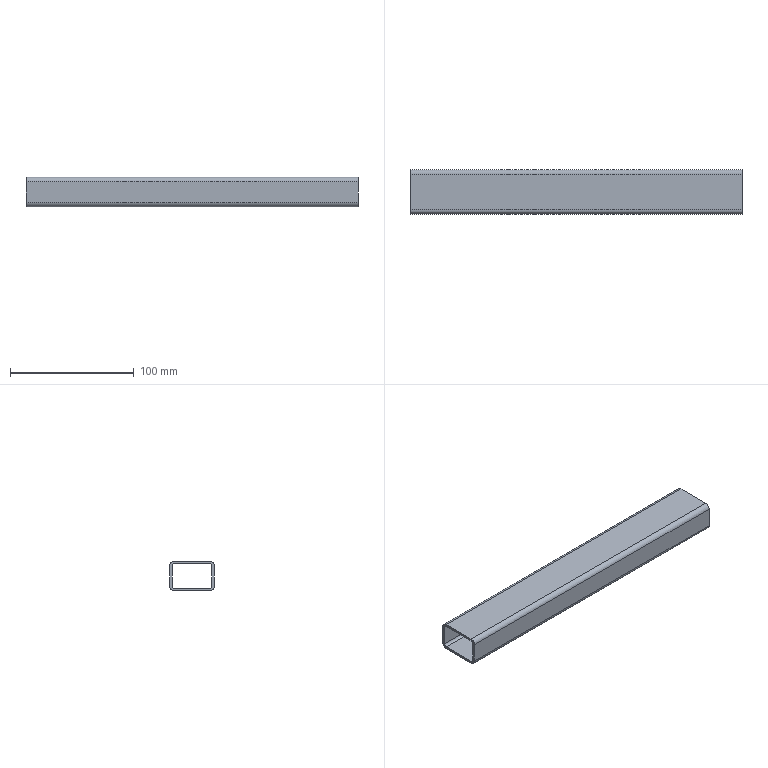Part | NX | 1 solid | 18 faces | box 268.32 x 36 x 24 mm | volume 55317 mm3 | plane 10 | cylinder 8 | commonest cylinder face diameters 3.84 x4 7.68 x4
STEP:
#1=CARTESIAN_POINT('',(264.834,-617.339,631.953));
#2=VERTEX_POINT('',#1);
#3=CARTESIAN_POINT('',(264.834,-613.499,628.113));
#4=VERTEX_POINT('',#3);
#5=CARTESIAN_POINT('',(264.834,-617.339,628.113));
#6=DIRECTION('',(-1.,0.,0.));
#7=DIRECTION('',(0.,0.,1.));
#8=AXIS2_PLACEMENT_3D('',#5,#6,#7);
#9=CIRCLE('',#8,3.84);
#10=EDGE_CURVE('',#2,#4,#9,.T.);
#11=ORIENTED_EDGE('',*,*,#10,.T.);
#12=CARTESIAN_POINT('',(-3.486,-613.499,628.113));
#13=VERTEX_POINT('',#12);
#14=CARTESIAN_POINT('',(-3.486,-613.499,628.113));
#15=DIRECTION('',(1.,0.,0.));
#16=VECTOR('',#15,1.);
#17=LINE('',#14,#16);
#18=EDGE_CURVE('',#13,#4,#17,.T.);
#19=ORIENTED_EDGE('',*,*,#18,.F.);
#20=CARTESIAN_POINT('',(-3.486,-617.339,631.953));
#21=VERTEX_POINT('',#20);
#22=CARTESIAN_POINT('',(-3.486,-617.339,628.113));
#23=DIRECTION('',(-1.,0.,0.));
#24=DIRECTION('',(0.,0.,1.));
#25=AXIS2_PLACEMENT_3D('',#22,#23,#24);
#26=CIRCLE('',#25,3.84);
#27=EDGE_CURVE('',#21,#13,#26,.T.);
#28=ORIENTED_EDGE('',*,*,#27,.F.);
#29=CARTESIAN_POINT('',(-3.486,-617.339,631.953));
#30=DIRECTION('',(1.,0.,0.));
#31=VECTOR('',#30,1.);
#32=LINE('',#29,#31);
#33=EDGE_CURVE('',#21,#2,#32,.T.);
#34=ORIENTED_EDGE('',*,*,#33,.T.);
#35=EDGE_LOOP('',(#11,#19,#28,#34));
#36=FACE_OUTER_BOUND('',#35,.T.);
#37=CARTESIAN_POINT('',(-3.486,-617.339,628.113));
#38=DIRECTION('',(1.,0.,0.));
#39=DIRECTION('',(0.,0.,-1.));
#40=AXIS2_PLACEMENT_3D('',#37,#38,#39);
#41=CYLINDRICAL_SURFACE('',#40,3.84);
#42=ADVANCED_FACE('',(#36),#41,.T.);
#43=CARTESIAN_POINT('',(264.834,-613.499,611.793));
#44=VERTEX_POINT('',#43);
#45=CARTESIAN_POINT('',(264.834,-613.499,628.113));
#46=DIRECTION('',(0.,0.,-1.));
#47=VECTOR('',#46,1.);
#48=LINE('',#45,#47);
#49=EDGE_CURVE('',#4,#44,#48,.T.);
#50=ORIENTED_EDGE('',*,*,#49,.T.);
#51=CARTESIAN_POINT('',(-3.486,-613.499,611.793));
#52=VERTEX_POINT('',#51);
#53=CARTESIAN_POINT('',(-3.486,-613.499,611.793));
#54=DIRECTION('',(1.,0.,0.));
#55=VECTOR('',#54,1.);
#56=LINE('',#53,#55);
#57=EDGE_CURVE('',#52,#44,#56,.T.);
#58=ORIENTED_EDGE('',*,*,#57,.F.);
#59=CARTESIAN_POINT('',(-3.486,-613.499,628.113));
#60=DIRECTION('',(0.,0.,-1.));
#61=VECTOR('',#60,1.);
#62=LINE('',#59,#61);
#63=EDGE_CURVE('',#13,#52,#62,.T.);
#64=ORIENTED_EDGE('',*,*,#63,.F.);
#65=ORIENTED_EDGE('',*,*,#18,.T.);
#66=EDGE_LOOP('',(#50,#58,#64,#65));
#67=FACE_OUTER_BOUND('',#66,.T.);
#68=CARTESIAN_POINT('',(-3.486,-613.499,628.113));
#69=DIRECTION('',(0.,-1.,0.));
#70=DIRECTION('',(0.,0.,-1.));
#71=AXIS2_PLACEMENT_3D('',#68,#69,#70);
#72=PLANE('',#71);
#73=ADVANCED_FACE('',(#67),#72,.F.);
#74=CARTESIAN_POINT('',(264.834,-617.339,607.953));
#75=VERTEX_POINT('',#74);
#76=CARTESIAN_POINT('',(264.834,-617.339,611.793));
#77=DIRECTION('',(-1.,0.,0.));
#78=DIRECTION('',(0.,0.,1.));
#79=AXIS2_PLACEMENT_3D('',#76,#77,#78);
#80=CIRCLE('',#79,3.84);
#81=EDGE_CURVE('',#44,#75,#80,.T.);
#82=ORIENTED_EDGE('',*,*,#81,.T.);
#83=CARTESIAN_POINT('',(-3.486,-617.339,607.953));
#84=VERTEX_POINT('',#83);
#85=CARTESIAN_POINT('',(-3.486,-617.339,607.953));
#86=DIRECTION('',(1.,0.,0.));
#87=VECTOR('',#86,1.);
#88=LINE('',#85,#87);
#89=EDGE_CURVE('',#84,#75,#88,.T.);
#90=ORIENTED_EDGE('',*,*,#89,.F.);
#91=CARTESIAN_POINT('',(-3.486,-617.339,611.793));
#92=DIRECTION('',(-1.,0.,0.));
#93=DIRECTION('',(0.,0.,1.));
#94=AXIS2_PLACEMENT_3D('',#91,#92,#93);
#95=CIRCLE('',#94,3.84);
#96=EDGE_CURVE('',#52,#84,#95,.T.);
#97=ORIENTED_EDGE('',*,*,#96,.F.);
#98=ORIENTED_EDGE('',*,*,#57,.T.);
#99=EDGE_LOOP('',(#82,#90,#97,#98));
#100=FACE_OUTER_BOUND('',#99,.T.);
#101=CARTESIAN_POINT('',(-3.486,-617.339,611.793));
#102=DIRECTION('',(1.,0.,0.));
#103=DIRECTION('',(0.,0.,-1.));
#104=AXIS2_PLACEMENT_3D('',#101,#102,#103);
#105=CYLINDRICAL_SURFACE('',#104,3.84);
#106=ADVANCED_FACE('',(#100),#105,.T.);
#107=CARTESIAN_POINT('',(264.834,-645.659,607.953));
#108=VERTEX_POINT('',#107);
#109=CARTESIAN_POINT('',(264.834,-645.659,607.953));
#110=DIRECTION('',(0.,-1.,0.));
#111=VECTOR('',#110,1.);
#112=LINE('',#109,#111);
#113=EDGE_CURVE('',#75,#108,#112,.T.);
#114=ORIENTED_EDGE('',*,*,#113,.T.);
#115=CARTESIAN_POINT('',(-3.486,-645.659,607.953));
#116=VERTEX_POINT('',#115);
#117=CARTESIAN_POINT('',(-3.486,-645.659,607.953));
#118=DIRECTION('',(1.,0.,0.));
#119=VECTOR('',#118,1.);
#120=LINE('',#117,#119);
#121=EDGE_CURVE('',#116,#108,#120,.T.);
#122=ORIENTED_EDGE('',*,*,#121,.F.);
#123=CARTESIAN_POINT('',(-3.486,-645.659,607.953));
#124=DIRECTION('',(0.,-1.,0.));
#125=VECTOR('',#124,1.);
#126=LINE('',#123,#125);
#127=EDGE_CURVE('',#84,#116,#126,.T.);
#128=ORIENTED_EDGE('',*,*,#127,.F.);
#129=ORIENTED_EDGE('',*,*,#89,.T.);
#130=EDGE_LOOP('',(#114,#122,#128,#129));
#131=FACE_OUTER_BOUND('',#130,.T.);
#132=CARTESIAN_POINT('',(-3.486,-645.659,607.953));
#133=DIRECTION('',(0.,0.,1.));
#134=DIRECTION('',(1.,0.,0.));
#135=AXIS2_PLACEMENT_3D('',#132,#133,#134);
#136=PLANE('',#135);
#137=ADVANCED_FACE('',(#131),#136,.F.);
#138=CARTESIAN_POINT('',(264.834,-649.499,611.793));
#139=VERTEX_POINT('',#138);
#140=CARTESIAN_POINT('',(264.834,-645.659,611.793));
#141=DIRECTION('',(-1.,0.,0.));
#142=DIRECTION('',(0.,0.,1.));
#143=AXIS2_PLACEMENT_3D('',#140,#141,#142);
#144=CIRCLE('',#143,3.84);
#145=EDGE_CURVE('',#108,#139,#144,.T.);
#146=ORIENTED_EDGE('',*,*,#145,.T.);
#147=CARTESIAN_POINT('',(-3.486,-649.499,611.793));
#148=VERTEX_POINT('',#147);
#149=CARTESIAN_POINT('',(-3.486,-649.499,611.793));
#150=DIRECTION('',(1.,0.,0.));
#151=VECTOR('',#150,1.);
#152=LINE('',#149,#151);
#153=EDGE_CURVE('',#148,#139,#152,.T.);
#154=ORIENTED_EDGE('',*,*,#153,.F.);
#155=CARTESIAN_POINT('',(-3.486,-645.659,611.793));
#156=DIRECTION('',(-1.,0.,0.));
#157=DIRECTION('',(0.,0.,1.));
#158=AXIS2_PLACEMENT_3D('',#155,#156,#157);
#159=CIRCLE('',#158,3.84);
#160=EDGE_CURVE('',#116,#148,#159,.T.);
#161=ORIENTED_EDGE('',*,*,#160,.F.);
#162=ORIENTED_EDGE('',*,*,#121,.T.);
#163=EDGE_LOOP('',(#146,#154,#161,#162));
#164=FACE_OUTER_BOUND('',#163,.T.);
#165=CARTESIAN_POINT('',(-3.486,-645.659,611.793));
#166=DIRECTION('',(1.,0.,0.));
#167=DIRECTION('',(0.,0.,-1.));
#168=AXIS2_PLACEMENT_3D('',#165,#166,#167);
#169=CYLINDRICAL_SURFACE('',#168,3.84);
#170=ADVANCED_FACE('',(#164),#169,.T.);
#171=CARTESIAN_POINT('',(264.834,-649.499,628.113));
#172=VERTEX_POINT('',#171);
#173=CARTESIAN_POINT('',(264.834,-649.499,611.793));
#174=DIRECTION('',(0.,0.,1.));
#175=VECTOR('',#174,1.);
#176=LINE('',#173,#175);
#177=EDGE_CURVE('',#139,#172,#176,.T.);
#178=ORIENTED_EDGE('',*,*,#177,.T.);
#179=CARTESIAN_POINT('',(-3.486,-649.499,628.113));
#180=VERTEX_POINT('',#179);
#181=CARTESIAN_POINT('',(-3.486,-649.499,628.113));
#182=DIRECTION('',(1.,0.,0.));
#183=VECTOR('',#182,1.);
#184=LINE('',#181,#183);
#185=EDGE_CURVE('',#180,#172,#184,.T.);
#186=ORIENTED_EDGE('',*,*,#185,.F.);
#187=CARTESIAN_POINT('',(-3.486,-649.499,611.793));
#188=DIRECTION('',(0.,0.,1.));
#189=VECTOR('',#188,1.);
#190=LINE('',#187,#189);
#191=EDGE_CURVE('',#148,#180,#190,.T.);
#192=ORIENTED_EDGE('',*,*,#191,.F.);
#193=ORIENTED_EDGE('',*,*,#153,.T.);
#194=EDGE_LOOP('',(#178,#186,#192,#193));
#195=FACE_OUTER_BOUND('',#194,.T.);
#196=CARTESIAN_POINT('',(-3.486,-649.499,611.793));
#197=DIRECTION('',(0.,1.,0.));
#198=DIRECTION('',(0.,0.,1.));
#199=AXIS2_PLACEMENT_3D('',#196,#197,#198);
#200=PLANE('',#199);
#201=ADVANCED_FACE('',(#195),#200,.F.);
#202=CARTESIAN_POINT('',(264.834,-645.659,631.953));
#203=VERTEX_POINT('',#202);
#204=CARTESIAN_POINT('',(264.834,-645.659,628.113));
#205=DIRECTION('',(-1.,0.,0.));
#206=DIRECTION('',(0.,0.,1.));
#207=AXIS2_PLACEMENT_3D('',#204,#205,#206);
#208=CIRCLE('',#207,3.84);
#209=EDGE_CURVE('',#172,#203,#208,.T.);
#210=ORIENTED_EDGE('',*,*,#209,.T.);
#211=CARTESIAN_POINT('',(-3.486,-645.659,631.953));
#212=VERTEX_POINT('',#211);
#213=CARTESIAN_POINT('',(-3.486,-645.659,631.953));
#214=DIRECTION('',(1.,0.,0.));
#215=VECTOR('',#214,1.);
#216=LINE('',#213,#215);
#217=EDGE_CURVE('',#212,#203,#216,.T.);
#218=ORIENTED_EDGE('',*,*,#217,.F.);
#219=CARTESIAN_POINT('',(-3.486,-645.659,628.113));
#220=DIRECTION('',(-1.,0.,0.));
#221=DIRECTION('',(0.,0.,1.));
#222=AXIS2_PLACEMENT_3D('',#219,#220,#221);
#223=CIRCLE('',#222,3.84);
#224=EDGE_CURVE('',#180,#212,#223,.T.);
#225=ORIENTED_EDGE('',*,*,#224,.F.);
#226=ORIENTED_EDGE('',*,*,#185,.T.);
#227=EDGE_LOOP('',(#210,#218,#225,#226));
#228=FACE_OUTER_BOUND('',#227,.T.);
#229=CARTESIAN_POINT('',(-3.486,-645.659,628.113));
#230=DIRECTION('',(1.,0.,0.));
#231=DIRECTION('',(0.,0.,-1.));
#232=AXIS2_PLACEMENT_3D('',#229,#230,#231);
#233=CYLINDRICAL_SURFACE('',#232,3.84);
#234=ADVANCED_FACE('',(#228),#233,.T.);
#235=CARTESIAN_POINT('',(264.834,-615.419,611.793));
#236=VERTEX_POINT('',#235);
#237=CARTESIAN_POINT('',(264.834,-617.339,609.873));
#238=VERTEX_POINT('',#237);
#239=CARTESIAN_POINT('',(264.834,-617.339,611.793));
#240=DIRECTION('',(-1.,0.,0.));
#241=DIRECTION('',(0.,0.,1.));
#242=AXIS2_PLACEMENT_3D('',#239,#240,#241);
#243=CIRCLE('',#242,1.92);
#244=EDGE_CURVE('',#236,#238,#243,.T.);
#245=ORIENTED_EDGE('',*,*,#244,.F.);
#246=CARTESIAN_POINT('',(-3.486,-615.419,611.793));
#247=VERTEX_POINT('',#246);
#248=CARTESIAN_POINT('',(-3.486,-615.419,611.793));
#249=DIRECTION('',(1.,0.,0.));
#250=VECTOR('',#249,1.);
#251=LINE('',#248,#250);
#252=EDGE_CURVE('',#247,#236,#251,.T.);
#253=ORIENTED_EDGE('',*,*,#252,.F.);
#254=CARTESIAN_POINT('',(-3.486,-617.339,609.873));
#255=VERTEX_POINT('',#254);
#256=CARTESIAN_POINT('',(-3.486,-617.339,611.793));
#257=DIRECTION('',(-1.,0.,0.));
#258=DIRECTION('',(0.,0.,1.));
#259=AXIS2_PLACEMENT_3D('',#256,#257,#258);
#260=CIRCLE('',#259,1.92);
#261=EDGE_CURVE('',#247,#255,#260,.T.);
#262=ORIENTED_EDGE('',*,*,#261,.T.);
#263=CARTESIAN_POINT('',(-3.486,-617.339,609.873));
#264=DIRECTION('',(1.,0.,0.));
#265=VECTOR('',#264,1.);
#266=LINE('',#263,#265);
#267=EDGE_CURVE('',#255,#238,#266,.T.);
#268=ORIENTED_EDGE('',*,*,#267,.T.);
#269=EDGE_LOOP('',(#245,#253,#262,#268));
#270=FACE_OUTER_BOUND('',#269,.T.);
#271=CARTESIAN_POINT('',(-3.486,-617.339,611.793));
#272=DIRECTION('',(1.,0.,0.));
#273=DIRECTION('',(0.,0.,-1.));
#274=AXIS2_PLACEMENT_3D('',#271,#272,#273);
#275=CYLINDRICAL_SURFACE('',#274,1.92);
#276=ADVANCED_FACE('',(#270),#275,.F.);
#277=CARTESIAN_POINT('',(264.834,-615.419,628.113));
#278=VERTEX_POINT('',#277);
#279=CARTESIAN_POINT('',(264.834,-615.419,628.113));
#280=DIRECTION('',(0.,0.,-1.));
#281=VECTOR('',#280,1.);
#282=LINE('',#279,#281);
#283=EDGE_CURVE('',#278,#236,#282,.T.);
#284=ORIENTED_EDGE('',*,*,#283,.F.);
#285=CARTESIAN_POINT('',(-3.486,-615.419,628.113));
#286=VERTEX_POINT('',#285);
#287=CARTESIAN_POINT('',(-3.486,-615.419,628.113));
#288=DIRECTION('',(1.,0.,0.));
#289=VECTOR('',#288,1.);
#290=LINE('',#287,#289);
#291=EDGE_CURVE('',#286,#278,#290,.T.);
#292=ORIENTED_EDGE('',*,*,#291,.F.);
#293=CARTESIAN_POINT('',(-3.486,-615.419,628.113));
#294=DIRECTION('',(0.,0.,-1.));
#295=VECTOR('',#294,1.);
#296=LINE('',#293,#295);
#297=EDGE_CURVE('',#286,#247,#296,.T.);
#298=ORIENTED_EDGE('',*,*,#297,.T.);
#299=ORIENTED_EDGE('',*,*,#252,.T.);
#300=EDGE_LOOP('',(#284,#292,#298,#299));
#301=FACE_OUTER_BOUND('',#300,.T.);
#302=CARTESIAN_POINT('',(-3.486,-615.419,628.113));
#303=DIRECTION('',(0.,-1.,0.));
#304=DIRECTION('',(0.,0.,-1.));
#305=AXIS2_PLACEMENT_3D('',#302,#303,#304);
#306=PLANE('',#305);
#307=ADVANCED_FACE('',(#301),#306,.T.);
#308=CARTESIAN_POINT('',(264.834,-617.339,630.033));
#309=VERTEX_POINT('',#308);
#310=CARTESIAN_POINT('',(264.834,-617.339,628.113));
#311=DIRECTION('',(-1.,0.,0.));
#312=DIRECTION('',(0.,0.,1.));
#313=AXIS2_PLACEMENT_3D('',#310,#311,#312);
#314=CIRCLE('',#313,1.92);
#315=EDGE_CURVE('',#309,#278,#314,.T.);
#316=ORIENTED_EDGE('',*,*,#315,.F.);
#317=CARTESIAN_POINT('',(-3.486,-617.339,630.033));
#318=VERTEX_POINT('',#317);
#319=CARTESIAN_POINT('',(-3.486,-617.339,630.033));
#320=DIRECTION('',(1.,0.,0.));
#321=VECTOR('',#320,1.);
#322=LINE('',#319,#321);
#323=EDGE_CURVE('',#318,#309,#322,.T.);
#324=ORIENTED_EDGE('',*,*,#323,.F.);
#325=CARTESIAN_POINT('',(-3.486,-617.339,628.113));
#326=DIRECTION('',(-1.,0.,0.));
#327=DIRECTION('',(0.,0.,1.));
#328=AXIS2_PLACEMENT_3D('',#325,#326,#327);
#329=CIRCLE('',#328,1.92);
#330=EDGE_CURVE('',#318,#286,#329,.T.);
#331=ORIENTED_EDGE('',*,*,#330,.T.);
#332=ORIENTED_EDGE('',*,*,#291,.T.);
#333=EDGE_LOOP('',(#316,#324,#331,#332));
#334=FACE_OUTER_BOUND('',#333,.T.);
#335=CARTESIAN_POINT('',(-3.486,-617.339,628.113));
#336=DIRECTION('',(1.,0.,0.));
#337=DIRECTION('',(0.,0.,-1.));
#338=AXIS2_PLACEMENT_3D('',#335,#336,#337);
#339=CYLINDRICAL_SURFACE('',#338,1.92);
#340=ADVANCED_FACE('',(#334),#339,.F.);
#341=CARTESIAN_POINT('',(264.834,-645.659,630.033));
#342=VERTEX_POINT('',#341);
#343=CARTESIAN_POINT('',(264.834,-617.339,630.033));
#344=DIRECTION('',(0.,1.,0.));
#345=VECTOR('',#344,1.);
#346=LINE('',#343,#345);
#347=EDGE_CURVE('',#342,#309,#346,.T.);
#348=ORIENTED_EDGE('',*,*,#347,.F.);
#349=CARTESIAN_POINT('',(-3.486,-645.659,630.033));
#350=VERTEX_POINT('',#349);
#351=CARTESIAN_POINT('',(-3.486,-645.659,630.033));
#352=DIRECTION('',(1.,0.,0.));
#353=VECTOR('',#352,1.);
#354=LINE('',#351,#353);
#355=EDGE_CURVE('',#350,#342,#354,.T.);
#356=ORIENTED_EDGE('',*,*,#355,.F.);
#357=CARTESIAN_POINT('',(-3.486,-617.339,630.033));
#358=DIRECTION('',(0.,1.,0.));
#359=VECTOR('',#358,1.);
#360=LINE('',#357,#359);
#361=EDGE_CURVE('',#350,#318,#360,.T.);
#362=ORIENTED_EDGE('',*,*,#361,.T.);
#363=ORIENTED_EDGE('',*,*,#323,.T.);
#364=EDGE_LOOP('',(#348,#356,#362,#363));
#365=FACE_OUTER_BOUND('',#364,.T.);
#366=CARTESIAN_POINT('',(-3.486,-617.339,630.033));
#367=DIRECTION('',(0.,0.,-1.));
#368=DIRECTION('',(-1.,0.,0.));
#369=AXIS2_PLACEMENT_3D('',#366,#367,#368);
#370=PLANE('',#369);
#371=ADVANCED_FACE('',(#365),#370,.T.);
#372=CARTESIAN_POINT('',(264.834,-647.579,628.113));
#373=VERTEX_POINT('',#372);
#374=CARTESIAN_POINT('',(264.834,-645.659,628.113));
#375=DIRECTION('',(-1.,0.,0.));
#376=DIRECTION('',(0.,0.,1.));
#377=AXIS2_PLACEMENT_3D('',#374,#375,#376);
#378=CIRCLE('',#377,1.92);
#379=EDGE_CURVE('',#373,#342,#378,.T.);
#380=ORIENTED_EDGE('',*,*,#379,.F.);
#381=CARTESIAN_POINT('',(-3.486,-647.579,628.113));
#382=VERTEX_POINT('',#381);
#383=CARTESIAN_POINT('',(-3.486,-647.579,628.113));
#384=DIRECTION('',(1.,0.,0.));
#385=VECTOR('',#384,1.);
#386=LINE('',#383,#385);
#387=EDGE_CURVE('',#382,#373,#386,.T.);
#388=ORIENTED_EDGE('',*,*,#387,.F.);
#389=CARTESIAN_POINT('',(-3.486,-645.659,628.113));
#390=DIRECTION('',(-1.,0.,0.));
#391=DIRECTION('',(0.,0.,1.));
#392=AXIS2_PLACEMENT_3D('',#389,#390,#391);
#393=CIRCLE('',#392,1.92);
#394=EDGE_CURVE('',#382,#350,#393,.T.);
#395=ORIENTED_EDGE('',*,*,#394,.T.);
#396=ORIENTED_EDGE('',*,*,#355,.T.);
#397=EDGE_LOOP('',(#380,#388,#395,#396));
#398=FACE_OUTER_BOUND('',#397,.T.);
#399=CARTESIAN_POINT('',(-3.486,-645.659,628.113));
#400=DIRECTION('',(1.,0.,0.));
#401=DIRECTION('',(0.,0.,-1.));
#402=AXIS2_PLACEMENT_3D('',#399,#400,#401);
#403=CYLINDRICAL_SURFACE('',#402,1.92);
#404=ADVANCED_FACE('',(#398),#403,.F.);
#405=CARTESIAN_POINT('',(264.834,-647.579,611.793));
#406=VERTEX_POINT('',#405);
#407=CARTESIAN_POINT('',(264.834,-647.579,611.793));
#408=DIRECTION('',(0.,0.,1.));
#409=VECTOR('',#408,1.);
#410=LINE('',#407,#409);
#411=EDGE_CURVE('',#406,#373,#410,.T.);
#412=ORIENTED_EDGE('',*,*,#411,.F.);
#413=CARTESIAN_POINT('',(-3.486,-647.579,611.793));
#414=VERTEX_POINT('',#413);
#415=CARTESIAN_POINT('',(-3.486,-647.579,611.793));
#416=DIRECTION('',(1.,0.,0.));
#417=VECTOR('',#416,1.);
#418=LINE('',#415,#417);
#419=EDGE_CURVE('',#414,#406,#418,.T.);
#420=ORIENTED_EDGE('',*,*,#419,.F.);
#421=CARTESIAN_POINT('',(-3.486,-647.579,611.793));
#422=DIRECTION('',(0.,0.,1.));
#423=VECTOR('',#422,1.);
#424=LINE('',#421,#423);
#425=EDGE_CURVE('',#414,#382,#424,.T.);
#426=ORIENTED_EDGE('',*,*,#425,.T.);
#427=ORIENTED_EDGE('',*,*,#387,.T.);
#428=EDGE_LOOP('',(#412,#420,#426,#427));
#429=FACE_OUTER_BOUND('',#428,.T.);
#430=CARTESIAN_POINT('',(-3.486,-647.579,611.793));
#431=DIRECTION('',(0.,1.,0.));
#432=DIRECTION('',(0.,0.,1.));
#433=AXIS2_PLACEMENT_3D('',#430,#431,#432);
#434=PLANE('',#433);
#435=ADVANCED_FACE('',(#429),#434,.T.);
#436=CARTESIAN_POINT('',(264.834,-645.659,609.873));
#437=VERTEX_POINT('',#436);
#438=CARTESIAN_POINT('',(264.834,-645.659,611.793));
#439=DIRECTION('',(-1.,0.,0.));
#440=DIRECTION('',(0.,0.,1.));
#441=AXIS2_PLACEMENT_3D('',#438,#439,#440);
#442=CIRCLE('',#441,1.92);
#443=EDGE_CURVE('',#437,#406,#442,.T.);
#444=ORIENTED_EDGE('',*,*,#443,.F.);
#445=CARTESIAN_POINT('',(-3.486,-645.659,609.873));
#446=VERTEX_POINT('',#445);
#447=CARTESIAN_POINT('',(-3.486,-645.659,609.873));
#448=DIRECTION('',(1.,0.,0.));
#449=VECTOR('',#448,1.);
#450=LINE('',#447,#449);
#451=EDGE_CURVE('',#446,#437,#450,.T.);
#452=ORIENTED_EDGE('',*,*,#451,.F.);
#453=CARTESIAN_POINT('',(-3.486,-645.659,611.793));
#454=DIRECTION('',(-1.,0.,0.));
#455=DIRECTION('',(0.,0.,1.));
#456=AXIS2_PLACEMENT_3D('',#453,#454,#455);
#457=CIRCLE('',#456,1.92);
#458=EDGE_CURVE('',#446,#414,#457,.T.);
#459=ORIENTED_EDGE('',*,*,#458,.T.);
#460=ORIENTED_EDGE('',*,*,#419,.T.);
#461=EDGE_LOOP('',(#444,#452,#459,#460));
#462=FACE_OUTER_BOUND('',#461,.T.);
#463=CARTESIAN_POINT('',(-3.486,-645.659,611.793));
#464=DIRECTION('',(1.,0.,0.));
#465=DIRECTION('',(0.,0.,-1.));
#466=AXIS2_PLACEMENT_3D('',#463,#464,#465);
#467=CYLINDRICAL_SURFACE('',#466,1.92);
#468=ADVANCED_FACE('',(#462),#467,.F.);
#469=CARTESIAN_POINT('',(264.834,-645.659,609.873));
#470=DIRECTION('',(0.,-1.,0.));
#471=VECTOR('',#470,1.);
#472=LINE('',#469,#471);
#473=EDGE_CURVE('',#238,#437,#472,.T.);
#474=ORIENTED_EDGE('',*,*,#473,.F.);
#475=ORIENTED_EDGE('',*,*,#267,.F.);
#476=CARTESIAN_POINT('',(-3.486,-645.659,609.873));
#477=DIRECTION('',(0.,-1.,0.));
#478=VECTOR('',#477,1.);
#479=LINE('',#476,#478);
#480=EDGE_CURVE('',#255,#446,#479,.T.);
#481=ORIENTED_EDGE('',*,*,#480,.T.);
#482=ORIENTED_EDGE('',*,*,#451,.T.);
#483=EDGE_LOOP('',(#474,#475,#481,#482));
#484=FACE_OUTER_BOUND('',#483,.T.);
#485=CARTESIAN_POINT('',(-3.486,-645.659,609.873));
#486=DIRECTION('',(0.,0.,1.));
#487=DIRECTION('',(1.,0.,0.));
#488=AXIS2_PLACEMENT_3D('',#485,#486,#487);
#489=PLANE('',#488);
#490=ADVANCED_FACE('',(#484),#489,.T.);
#491=CARTESIAN_POINT('',(264.834,-617.339,631.953));
#492=DIRECTION('',(0.,1.,0.));
#493=VECTOR('',#492,1.);
#494=LINE('',#491,#493);
#495=EDGE_CURVE('',#203,#2,#494,.T.);
#496=ORIENTED_EDGE('',*,*,#495,.T.);
#497=ORIENTED_EDGE('',*,*,#33,.F.);
#498=CARTESIAN_POINT('',(-3.486,-617.339,631.953));
#499=DIRECTION('',(0.,1.,0.));
#500=VECTOR('',#499,1.);
#501=LINE('',#498,#500);
#502=EDGE_CURVE('',#212,#21,#501,.T.);
#503=ORIENTED_EDGE('',*,*,#502,.F.);
#504=ORIENTED_EDGE('',*,*,#217,.T.);
#505=EDGE_LOOP('',(#496,#497,#503,#504));
#506=FACE_OUTER_BOUND('',#505,.T.);
#507=CARTESIAN_POINT('',(-3.486,-617.339,631.953));
#508=DIRECTION('',(0.,0.,-1.));
#509=DIRECTION('',(-1.,0.,0.));
#510=AXIS2_PLACEMENT_3D('',#507,#508,#509);
#511=PLANE('',#510);
#512=ADVANCED_FACE('',(#506),#511,.F.);
#513=ORIENTED_EDGE('',*,*,#261,.F.);
#514=ORIENTED_EDGE('',*,*,#297,.F.);
#515=ORIENTED_EDGE('',*,*,#330,.F.);
#516=ORIENTED_EDGE('',*,*,#361,.F.);
#517=ORIENTED_EDGE('',*,*,#394,.F.);
#518=ORIENTED_EDGE('',*,*,#425,.F.);
#519=ORIENTED_EDGE('',*,*,#458,.F.);
#520=ORIENTED_EDGE('',*,*,#480,.F.);
#521=EDGE_LOOP('',(#513,#514,#515,#516,#517,#518,#519,#520));
#522=FACE_BOUND('',#521,.T.);
#523=ORIENTED_EDGE('',*,*,#27,.T.);
#524=ORIENTED_EDGE('',*,*,#63,.T.);
#525=ORIENTED_EDGE('',*,*,#96,.T.);
#526=ORIENTED_EDGE('',*,*,#127,.T.);
#527=ORIENTED_EDGE('',*,*,#160,.T.);
#528=ORIENTED_EDGE('',*,*,#191,.T.);
#529=ORIENTED_EDGE('',*,*,#224,.T.);
#530=ORIENTED_EDGE('',*,*,#502,.T.);
#531=EDGE_LOOP('',(#523,#524,#525,#526,#527,#528,#529,#530));
#532=FACE_BOUND('',#531,.T.);
#533=CARTESIAN_POINT('',(-3.486,-617.339,628.113));
#534=DIRECTION('',(-1.,0.,0.));
#535=DIRECTION('',(0.,0.,1.));
#536=AXIS2_PLACEMENT_3D('',#533,#534,#535);
#537=PLANE('',#536);
#538=ADVANCED_FACE('',(#522,#532),#537,.T.);
#539=ORIENTED_EDGE('',*,*,#244,.T.);
#540=ORIENTED_EDGE('',*,*,#473,.T.);
#541=ORIENTED_EDGE('',*,*,#443,.T.);
#542=ORIENTED_EDGE('',*,*,#411,.T.);
#543=ORIENTED_EDGE('',*,*,#379,.T.);
#544=ORIENTED_EDGE('',*,*,#347,.T.);
#545=ORIENTED_EDGE('',*,*,#315,.T.);
#546=ORIENTED_EDGE('',*,*,#283,.T.);
#547=EDGE_LOOP('',(#539,#540,#541,#542,#543,#544,#545,#546));
#548=FACE_BOUND('',#547,.T.);
#549=ORIENTED_EDGE('',*,*,#10,.F.);
#550=ORIENTED_EDGE('',*,*,#495,.F.);
#551=ORIENTED_EDGE('',*,*,#209,.F.);
#552=ORIENTED_EDGE('',*,*,#177,.F.);
#553=ORIENTED_EDGE('',*,*,#145,.F.);
#554=ORIENTED_EDGE('',*,*,#113,.F.);
#555=ORIENTED_EDGE('',*,*,#81,.F.);
#556=ORIENTED_EDGE('',*,*,#49,.F.);
#557=EDGE_LOOP('',(#549,#550,#551,#552,#553,#554,#555,#556));
#558=FACE_BOUND('',#557,.T.);
#559=CARTESIAN_POINT('',(264.834,-617.339,628.113));
#560=DIRECTION('',(-1.,0.,0.));
#561=DIRECTION('',(0.,0.,1.));
#562=AXIS2_PLACEMENT_3D('',#559,#560,#561);
#563=PLANE('',#562);
#564=ADVANCED_FACE('',(#548,#558),#563,.F.);
#565=CLOSED_SHELL('',(#42,#73,#106,#137,#170,#201,#234,#276,#307,#340,#371,#404,#435,#468,#490,#512,#538,#564));
#566=MANIFOLD_SOLID_BREP('',#565);
#567=(LENGTH_UNIT()NAMED_UNIT(*)SI_UNIT(.MILLI.,.METRE.));
#568=UNCERTAINTY_MEASURE_WITH_UNIT(LENGTH_MEASURE(0.00002),#567,'','');
#569=(NAMED_UNIT(*)PLANE_ANGLE_UNIT()SI_UNIT($,.RADIAN.));
#570=PLANE_ANGLE_MEASURE_WITH_UNIT(PLANE_ANGLE_MEASURE(0.01745),#569);
#571=DIMENSIONAL_EXPONENTS(0.,0.,0.,0.,0.,0.,0.);
#572=(CONVERSION_BASED_UNIT('DEGREE',#570)NAMED_UNIT(#571)PLANE_ANGLE_UNIT());
#573=(NAMED_UNIT(*)SI_UNIT($,.STERADIAN.)SOLID_ANGLE_UNIT());
#574=(GEOMETRIC_REPRESENTATION_CONTEXT(3)GLOBAL_UNCERTAINTY_ASSIGNED_CONTEXT((#568))GLOBAL_UNIT_ASSIGNED_CONTEXT((#567,#572,#573))REPRESENTATION_CONTEXT('',''));
#575=ADVANCED_BREP_SHAPE_REPRESENTATION('',(#566),#574);